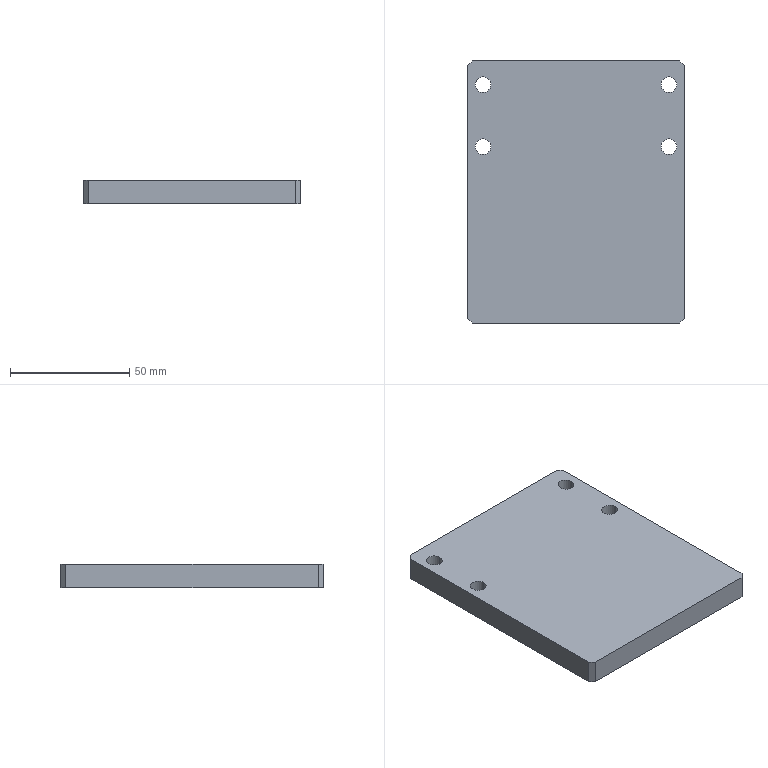Part | SolidWorks | features BaseBody 1 | 1 solid | 18 faces | box 91 x 110 x 10 mm | volume 98652 mm3 | plane 10 | cylinder 8 | commonest cylinder face diameters 6.6 x8
STEP:
#1=CARTESIAN_POINT('',(-42.3,19.,0.));
#2=VERTEX_POINT('',#1);
#3=CARTESIAN_POINT('',(-35.7,19.,0.));
#4=VERTEX_POINT('',#3);
#5=CARTESIAN_POINT('',(-39.,19.,0.));
#6=DIRECTION('',(0.,0.,1.));
#7=DIRECTION('',(1.,0.,0.));
#8=AXIS2_PLACEMENT_3D('',#5,#6,#7);
#9=CIRCLE('',#8,3.3);
#10=EDGE_CURVE('',#2,#4,#9,.T.);
#11=ORIENTED_EDGE('',*,*,#10,.F.);
#12=CARTESIAN_POINT('',(-42.3,19.,10.));
#13=VERTEX_POINT('',#12);
#14=CARTESIAN_POINT('',(-42.3,19.,10.));
#15=DIRECTION('',(0.,0.,1.));
#16=VECTOR('',#15,1000.);
#17=LINE('',#14,#16);
#18=EDGE_CURVE('',#2,#13,#17,.T.);
#19=ORIENTED_EDGE('',*,*,#18,.T.);
#20=CARTESIAN_POINT('',(-35.7,19.,10.));
#21=VERTEX_POINT('',#20);
#22=CARTESIAN_POINT('',(-39.,19.,10.));
#23=DIRECTION('',(0.,0.,-1.));
#24=DIRECTION('',(1.,0.,0.));
#25=AXIS2_PLACEMENT_3D('',#22,#23,#24);
#26=CIRCLE('',#25,3.3);
#27=EDGE_CURVE('',#21,#13,#26,.T.);
#28=ORIENTED_EDGE('',*,*,#27,.F.);
#29=CARTESIAN_POINT('',(-35.7,19.,10.));
#30=DIRECTION('',(0.,0.,1.));
#31=VECTOR('',#30,1000.);
#32=LINE('',#29,#31);
#33=EDGE_CURVE('',#4,#21,#32,.T.);
#34=ORIENTED_EDGE('',*,*,#33,.F.);
#35=EDGE_LOOP('',(#11,#19,#28,#34));
#36=FACE_OUTER_BOUND('',#35,.T.);
#37=CARTESIAN_POINT('',(-39.,19.,10.));
#38=DIRECTION('',(0.,0.,1.));
#39=DIRECTION('',(1.,0.,0.));
#40=AXIS2_PLACEMENT_3D('',#37,#38,#39);
#41=CYLINDRICAL_SURFACE('',#40,3.3);
#42=ADVANCED_FACE('',(#36),#41,.F.);
#43=CARTESIAN_POINT('',(35.7,19.,0.));
#44=VERTEX_POINT('',#43);
#45=CARTESIAN_POINT('',(42.3,19.,0.));
#46=VERTEX_POINT('',#45);
#47=CARTESIAN_POINT('',(39.,19.,0.));
#48=DIRECTION('',(0.,0.,1.));
#49=DIRECTION('',(1.,0.,0.));
#50=AXIS2_PLACEMENT_3D('',#47,#48,#49);
#51=CIRCLE('',#50,3.3);
#52=EDGE_CURVE('',#44,#46,#51,.T.);
#53=ORIENTED_EDGE('',*,*,#52,.F.);
#54=CARTESIAN_POINT('',(35.7,19.,10.));
#55=VERTEX_POINT('',#54);
#56=CARTESIAN_POINT('',(35.7,19.,10.));
#57=DIRECTION('',(0.,0.,1.));
#58=VECTOR('',#57,1000.);
#59=LINE('',#56,#58);
#60=EDGE_CURVE('',#44,#55,#59,.T.);
#61=ORIENTED_EDGE('',*,*,#60,.T.);
#62=CARTESIAN_POINT('',(42.3,19.,10.));
#63=VERTEX_POINT('',#62);
#64=CARTESIAN_POINT('',(39.,19.,10.));
#65=DIRECTION('',(0.,0.,-1.));
#66=DIRECTION('',(1.,0.,0.));
#67=AXIS2_PLACEMENT_3D('',#64,#65,#66);
#68=CIRCLE('',#67,3.3);
#69=EDGE_CURVE('',#63,#55,#68,.T.);
#70=ORIENTED_EDGE('',*,*,#69,.F.);
#71=CARTESIAN_POINT('',(42.3,19.,10.));
#72=DIRECTION('',(0.,0.,1.));
#73=VECTOR('',#72,1000.);
#74=LINE('',#71,#73);
#75=EDGE_CURVE('',#46,#63,#74,.T.);
#76=ORIENTED_EDGE('',*,*,#75,.F.);
#77=EDGE_LOOP('',(#53,#61,#70,#76));
#78=FACE_OUTER_BOUND('',#77,.T.);
#79=CARTESIAN_POINT('',(39.,19.,10.));
#80=DIRECTION('',(0.,0.,1.));
#81=DIRECTION('',(1.,0.,0.));
#82=AXIS2_PLACEMENT_3D('',#79,#80,#81);
#83=CYLINDRICAL_SURFACE('',#82,3.3);
#84=ADVANCED_FACE('',(#78),#83,.F.);
#85=CARTESIAN_POINT('',(35.7,45.,0.));
#86=VERTEX_POINT('',#85);
#87=CARTESIAN_POINT('',(42.3,45.,0.));
#88=VERTEX_POINT('',#87);
#89=CARTESIAN_POINT('',(39.,45.,0.));
#90=DIRECTION('',(0.,0.,1.));
#91=DIRECTION('',(1.,0.,0.));
#92=AXIS2_PLACEMENT_3D('',#89,#90,#91);
#93=CIRCLE('',#92,3.3);
#94=EDGE_CURVE('',#86,#88,#93,.T.);
#95=ORIENTED_EDGE('',*,*,#94,.F.);
#96=CARTESIAN_POINT('',(35.7,45.,10.));
#97=VERTEX_POINT('',#96);
#98=CARTESIAN_POINT('',(35.7,45.,10.));
#99=DIRECTION('',(0.,0.,1.));
#100=VECTOR('',#99,1000.);
#101=LINE('',#98,#100);
#102=EDGE_CURVE('',#86,#97,#101,.T.);
#103=ORIENTED_EDGE('',*,*,#102,.T.);
#104=CARTESIAN_POINT('',(42.3,45.,10.));
#105=VERTEX_POINT('',#104);
#106=CARTESIAN_POINT('',(39.,45.,10.));
#107=DIRECTION('',(0.,0.,-1.));
#108=DIRECTION('',(1.,0.,0.));
#109=AXIS2_PLACEMENT_3D('',#106,#107,#108);
#110=CIRCLE('',#109,3.3);
#111=EDGE_CURVE('',#105,#97,#110,.T.);
#112=ORIENTED_EDGE('',*,*,#111,.F.);
#113=CARTESIAN_POINT('',(42.3,45.,10.));
#114=DIRECTION('',(0.,0.,1.));
#115=VECTOR('',#114,1000.);
#116=LINE('',#113,#115);
#117=EDGE_CURVE('',#88,#105,#116,.T.);
#118=ORIENTED_EDGE('',*,*,#117,.F.);
#119=EDGE_LOOP('',(#95,#103,#112,#118));
#120=FACE_OUTER_BOUND('',#119,.T.);
#121=CARTESIAN_POINT('',(39.,45.,10.));
#122=DIRECTION('',(0.,0.,1.));
#123=DIRECTION('',(1.,0.,0.));
#124=AXIS2_PLACEMENT_3D('',#121,#122,#123);
#125=CYLINDRICAL_SURFACE('',#124,3.3);
#126=ADVANCED_FACE('',(#120),#125,.F.);
#127=CARTESIAN_POINT('',(-42.3,45.,0.));
#128=VERTEX_POINT('',#127);
#129=CARTESIAN_POINT('',(-35.7,45.,0.));
#130=VERTEX_POINT('',#129);
#131=CARTESIAN_POINT('',(-39.,45.,0.));
#132=DIRECTION('',(0.,0.,1.));
#133=DIRECTION('',(1.,0.,0.));
#134=AXIS2_PLACEMENT_3D('',#131,#132,#133);
#135=CIRCLE('',#134,3.3);
#136=EDGE_CURVE('',#128,#130,#135,.T.);
#137=ORIENTED_EDGE('',*,*,#136,.F.);
#138=CARTESIAN_POINT('',(-42.3,45.,10.));
#139=VERTEX_POINT('',#138);
#140=CARTESIAN_POINT('',(-42.3,45.,10.));
#141=DIRECTION('',(0.,0.,1.));
#142=VECTOR('',#141,1000.);
#143=LINE('',#140,#142);
#144=EDGE_CURVE('',#128,#139,#143,.T.);
#145=ORIENTED_EDGE('',*,*,#144,.T.);
#146=CARTESIAN_POINT('',(-35.7,45.,10.));
#147=VERTEX_POINT('',#146);
#148=CARTESIAN_POINT('',(-39.,45.,10.));
#149=DIRECTION('',(0.,0.,-1.));
#150=DIRECTION('',(1.,0.,0.));
#151=AXIS2_PLACEMENT_3D('',#148,#149,#150);
#152=CIRCLE('',#151,3.3);
#153=EDGE_CURVE('',#147,#139,#152,.T.);
#154=ORIENTED_EDGE('',*,*,#153,.F.);
#155=CARTESIAN_POINT('',(-35.7,45.,10.));
#156=DIRECTION('',(0.,0.,1.));
#157=VECTOR('',#156,1000.);
#158=LINE('',#155,#157);
#159=EDGE_CURVE('',#130,#147,#158,.T.);
#160=ORIENTED_EDGE('',*,*,#159,.F.);
#161=EDGE_LOOP('',(#137,#145,#154,#160));
#162=FACE_OUTER_BOUND('',#161,.T.);
#163=CARTESIAN_POINT('',(-39.,45.,10.));
#164=DIRECTION('',(0.,0.,1.));
#165=DIRECTION('',(1.,0.,0.));
#166=AXIS2_PLACEMENT_3D('',#163,#164,#165);
#167=CYLINDRICAL_SURFACE('',#166,3.3);
#168=ADVANCED_FACE('',(#162),#167,.F.);
#169=CARTESIAN_POINT('',(43.5,55.,10.));
#170=VERTEX_POINT('',#169);
#171=CARTESIAN_POINT('',(-43.5,55.,10.));
#172=VERTEX_POINT('',#171);
#173=CARTESIAN_POINT('',(0.,55.,10.));
#174=DIRECTION('',(-1.,0.,0.));
#175=VECTOR('',#174,1000.);
#176=LINE('',#173,#175);
#177=EDGE_CURVE('',#170,#172,#176,.T.);
#178=ORIENTED_EDGE('',*,*,#177,.T.);
#179=CARTESIAN_POINT('',(-45.5,53.,10.));
#180=VERTEX_POINT('',#179);
#181=CARTESIAN_POINT('',(-43.5,55.,10.));
#182=DIRECTION('',(-0.7071,-0.7071,0.));
#183=VECTOR('',#182,1000.);
#184=LINE('',#181,#183);
#185=EDGE_CURVE('',#172,#180,#184,.T.);
#186=ORIENTED_EDGE('',*,*,#185,.T.);
#187=CARTESIAN_POINT('',(-45.5,-53.,10.));
#188=VERTEX_POINT('',#187);
#189=CARTESIAN_POINT('',(-45.5,0.,10.));
#190=DIRECTION('',(0.,-1.,0.));
#191=VECTOR('',#190,1000.);
#192=LINE('',#189,#191);
#193=EDGE_CURVE('',#180,#188,#192,.T.);
#194=ORIENTED_EDGE('',*,*,#193,.T.);
#195=CARTESIAN_POINT('',(-43.5,-55.,10.));
#196=VERTEX_POINT('',#195);
#197=CARTESIAN_POINT('',(-45.5,-53.,10.));
#198=DIRECTION('',(0.7071,-0.7071,0.));
#199=VECTOR('',#198,1000.);
#200=LINE('',#197,#199);
#201=EDGE_CURVE('',#188,#196,#200,.T.);
#202=ORIENTED_EDGE('',*,*,#201,.T.);
#203=CARTESIAN_POINT('',(43.5,-55.,10.));
#204=VERTEX_POINT('',#203);
#205=CARTESIAN_POINT('',(0.,-55.,10.));
#206=DIRECTION('',(1.,0.,0.));
#207=VECTOR('',#206,1000.);
#208=LINE('',#205,#207);
#209=EDGE_CURVE('',#196,#204,#208,.T.);
#210=ORIENTED_EDGE('',*,*,#209,.T.);
#211=CARTESIAN_POINT('',(45.5,-53.,10.));
#212=VERTEX_POINT('',#211);
#213=CARTESIAN_POINT('',(43.5,-55.,10.));
#214=DIRECTION('',(0.7071,0.7071,0.));
#215=VECTOR('',#214,1000.);
#216=LINE('',#213,#215);
#217=EDGE_CURVE('',#204,#212,#216,.T.);
#218=ORIENTED_EDGE('',*,*,#217,.T.);
#219=CARTESIAN_POINT('',(45.5,53.,10.));
#220=VERTEX_POINT('',#219);
#221=CARTESIAN_POINT('',(45.5,0.,10.));
#222=DIRECTION('',(0.,1.,0.));
#223=VECTOR('',#222,1000.);
#224=LINE('',#221,#223);
#225=EDGE_CURVE('',#212,#220,#224,.T.);
#226=ORIENTED_EDGE('',*,*,#225,.T.);
#227=CARTESIAN_POINT('',(45.5,53.,10.));
#228=DIRECTION('',(-0.7071,0.7071,0.));
#229=VECTOR('',#228,1000.);
#230=LINE('',#227,#229);
#231=EDGE_CURVE('',#220,#170,#230,.T.);
#232=ORIENTED_EDGE('',*,*,#231,.T.);
#233=EDGE_LOOP('',(#178,#186,#194,#202,#210,#218,#226,#232));
#234=FACE_OUTER_BOUND('',#233,.T.);
#235=ORIENTED_EDGE('',*,*,#27,.T.);
#236=CARTESIAN_POINT('',(-39.,19.,10.));
#237=DIRECTION('',(0.,0.,-1.));
#238=DIRECTION('',(1.,0.,0.));
#239=AXIS2_PLACEMENT_3D('',#236,#237,#238);
#240=CIRCLE('',#239,3.3);
#241=EDGE_CURVE('',#13,#21,#240,.T.);
#242=ORIENTED_EDGE('',*,*,#241,.T.);
#243=EDGE_LOOP('',(#235,#242));
#244=FACE_BOUND('',#243,.T.);
#245=ORIENTED_EDGE('',*,*,#69,.T.);
#246=CARTESIAN_POINT('',(39.,19.,10.));
#247=DIRECTION('',(0.,0.,-1.));
#248=DIRECTION('',(1.,0.,0.));
#249=AXIS2_PLACEMENT_3D('',#246,#247,#248);
#250=CIRCLE('',#249,3.3);
#251=EDGE_CURVE('',#55,#63,#250,.T.);
#252=ORIENTED_EDGE('',*,*,#251,.T.);
#253=EDGE_LOOP('',(#245,#252));
#254=FACE_BOUND('',#253,.T.);
#255=ORIENTED_EDGE('',*,*,#111,.T.);
#256=CARTESIAN_POINT('',(39.,45.,10.));
#257=DIRECTION('',(0.,0.,-1.));
#258=DIRECTION('',(1.,0.,0.));
#259=AXIS2_PLACEMENT_3D('',#256,#257,#258);
#260=CIRCLE('',#259,3.3);
#261=EDGE_CURVE('',#97,#105,#260,.T.);
#262=ORIENTED_EDGE('',*,*,#261,.T.);
#263=EDGE_LOOP('',(#255,#262));
#264=FACE_BOUND('',#263,.T.);
#265=ORIENTED_EDGE('',*,*,#153,.T.);
#266=CARTESIAN_POINT('',(-39.,45.,10.));
#267=DIRECTION('',(0.,0.,-1.));
#268=DIRECTION('',(1.,0.,0.));
#269=AXIS2_PLACEMENT_3D('',#266,#267,#268);
#270=CIRCLE('',#269,3.3);
#271=EDGE_CURVE('',#139,#147,#270,.T.);
#272=ORIENTED_EDGE('',*,*,#271,.T.);
#273=EDGE_LOOP('',(#265,#272));
#274=FACE_BOUND('',#273,.T.);
#275=CARTESIAN_POINT('',(0.,0.,10.));
#276=DIRECTION('',(0.,0.,1.));
#277=DIRECTION('',(1.,0.,0.));
#278=AXIS2_PLACEMENT_3D('',#275,#276,#277);
#279=PLANE('',#278);
#280=ADVANCED_FACE('',(#234,#244,#254,#264,#274),#279,.T.);
#281=CARTESIAN_POINT('',(-43.5,55.,0.));
#282=VERTEX_POINT('',#281);
#283=CARTESIAN_POINT('',(-43.5,55.,10.));
#284=DIRECTION('',(0.,0.,1.));
#285=VECTOR('',#284,1000.);
#286=LINE('',#283,#285);
#287=EDGE_CURVE('',#282,#172,#286,.T.);
#288=ORIENTED_EDGE('',*,*,#287,.F.);
#289=CARTESIAN_POINT('',(-45.5,53.,0.));
#290=VERTEX_POINT('',#289);
#291=CARTESIAN_POINT('',(-45.5,53.,0.));
#292=DIRECTION('',(0.7071,0.7071,0.));
#293=VECTOR('',#292,1000.);
#294=LINE('',#291,#293);
#295=EDGE_CURVE('',#290,#282,#294,.T.);
#296=ORIENTED_EDGE('',*,*,#295,.F.);
#297=CARTESIAN_POINT('',(-45.5,53.,10.));
#298=DIRECTION('',(0.,0.,-1.));
#299=VECTOR('',#298,1000.);
#300=LINE('',#297,#299);
#301=EDGE_CURVE('',#180,#290,#300,.T.);
#302=ORIENTED_EDGE('',*,*,#301,.F.);
#303=ORIENTED_EDGE('',*,*,#185,.F.);
#304=EDGE_LOOP('',(#288,#296,#302,#303));
#305=FACE_OUTER_BOUND('',#304,.T.);
#306=CARTESIAN_POINT('',(-45.5,53.,10.));
#307=DIRECTION('',(0.7071,-0.7071,0.));
#308=DIRECTION('',(0.7071,0.7071,0.));
#309=AXIS2_PLACEMENT_3D('',#306,#307,#308);
#310=PLANE('',#309);
#311=ADVANCED_FACE('',(#305),#310,.F.);
#312=CARTESIAN_POINT('',(43.5,55.,0.));
#313=VERTEX_POINT('',#312);
#314=CARTESIAN_POINT('',(43.5,55.,10.));
#315=DIRECTION('',(0.,0.,1.));
#316=VECTOR('',#315,1000.);
#317=LINE('',#314,#316);
#318=EDGE_CURVE('',#313,#170,#317,.T.);
#319=ORIENTED_EDGE('',*,*,#318,.F.);
#320=CARTESIAN_POINT('',(-45.5,55.,0.));
#321=DIRECTION('',(1.,0.,0.));
#322=VECTOR('',#321,1000.);
#323=LINE('',#320,#322);
#324=EDGE_CURVE('',#282,#313,#323,.T.);
#325=ORIENTED_EDGE('',*,*,#324,.F.);
#326=ORIENTED_EDGE('',*,*,#287,.T.);
#327=ORIENTED_EDGE('',*,*,#177,.F.);
#328=EDGE_LOOP('',(#319,#325,#326,#327));
#329=FACE_OUTER_BOUND('',#328,.T.);
#330=CARTESIAN_POINT('',(-45.5,55.,10.));
#331=DIRECTION('',(0.,-1.,0.));
#332=DIRECTION('',(0.,0.,-1.));
#333=AXIS2_PLACEMENT_3D('',#330,#331,#332);
#334=PLANE('',#333);
#335=ADVANCED_FACE('',(#329),#334,.F.);
#336=CARTESIAN_POINT('',(45.5,53.,0.));
#337=VERTEX_POINT('',#336);
#338=CARTESIAN_POINT('',(45.5,53.,10.));
#339=DIRECTION('',(0.,0.,1.));
#340=VECTOR('',#339,1000.);
#341=LINE('',#338,#340);
#342=EDGE_CURVE('',#337,#220,#341,.T.);
#343=ORIENTED_EDGE('',*,*,#342,.F.);
#344=CARTESIAN_POINT('',(43.5,55.,0.));
#345=DIRECTION('',(0.7071,-0.7071,0.));
#346=VECTOR('',#345,1000.);
#347=LINE('',#344,#346);
#348=EDGE_CURVE('',#313,#337,#347,.T.);
#349=ORIENTED_EDGE('',*,*,#348,.F.);
#350=ORIENTED_EDGE('',*,*,#318,.T.);
#351=ORIENTED_EDGE('',*,*,#231,.F.);
#352=EDGE_LOOP('',(#343,#349,#350,#351));
#353=FACE_OUTER_BOUND('',#352,.T.);
#354=CARTESIAN_POINT('',(43.5,55.,10.));
#355=DIRECTION('',(-0.7071,-0.7071,0.));
#356=DIRECTION('',(0.7071,-0.7071,0.));
#357=AXIS2_PLACEMENT_3D('',#354,#355,#356);
#358=PLANE('',#357);
#359=ADVANCED_FACE('',(#353),#358,.F.);
#360=CARTESIAN_POINT('',(45.5,-53.,0.));
#361=VERTEX_POINT('',#360);
#362=CARTESIAN_POINT('',(45.5,-53.,10.));
#363=DIRECTION('',(0.,0.,1.));
#364=VECTOR('',#363,1000.);
#365=LINE('',#362,#364);
#366=EDGE_CURVE('',#361,#212,#365,.T.);
#367=ORIENTED_EDGE('',*,*,#366,.F.);
#368=CARTESIAN_POINT('',(45.5,55.,0.));
#369=DIRECTION('',(0.,-1.,0.));
#370=VECTOR('',#369,1000.);
#371=LINE('',#368,#370);
#372=EDGE_CURVE('',#337,#361,#371,.T.);
#373=ORIENTED_EDGE('',*,*,#372,.F.);
#374=ORIENTED_EDGE('',*,*,#342,.T.);
#375=ORIENTED_EDGE('',*,*,#225,.F.);
#376=EDGE_LOOP('',(#367,#373,#374,#375));
#377=FACE_OUTER_BOUND('',#376,.T.);
#378=CARTESIAN_POINT('',(45.5,55.,10.));
#379=DIRECTION('',(-1.,0.,0.));
#380=DIRECTION('',(0.,-1.,0.));
#381=AXIS2_PLACEMENT_3D('',#378,#379,#380);
#382=PLANE('',#381);
#383=ADVANCED_FACE('',(#377),#382,.F.);
#384=CARTESIAN_POINT('',(43.5,-55.,0.));
#385=VERTEX_POINT('',#384);
#386=CARTESIAN_POINT('',(43.5,-55.,10.));
#387=DIRECTION('',(0.,0.,1.));
#388=VECTOR('',#387,1000.);
#389=LINE('',#386,#388);
#390=EDGE_CURVE('',#385,#204,#389,.T.);
#391=ORIENTED_EDGE('',*,*,#390,.F.);
#392=CARTESIAN_POINT('',(45.5,-53.,0.));
#393=DIRECTION('',(-0.7071,-0.7071,0.));
#394=VECTOR('',#393,1000.);
#395=LINE('',#392,#394);
#396=EDGE_CURVE('',#361,#385,#395,.T.);
#397=ORIENTED_EDGE('',*,*,#396,.F.);
#398=ORIENTED_EDGE('',*,*,#366,.T.);
#399=ORIENTED_EDGE('',*,*,#217,.F.);
#400=EDGE_LOOP('',(#391,#397,#398,#399));
#401=FACE_OUTER_BOUND('',#400,.T.);
#402=CARTESIAN_POINT('',(45.5,-53.,10.));
#403=DIRECTION('',(-0.7071,0.7071,0.));
#404=DIRECTION('',(-0.7071,-0.7071,0.));
#405=AXIS2_PLACEMENT_3D('',#402,#403,#404);
#406=PLANE('',#405);
#407=ADVANCED_FACE('',(#401),#406,.F.);
#408=CARTESIAN_POINT('',(-43.5,-55.,0.));
#409=VERTEX_POINT('',#408);
#410=CARTESIAN_POINT('',(-43.5,-55.,10.));
#411=DIRECTION('',(0.,0.,1.));
#412=VECTOR('',#411,1000.);
#413=LINE('',#410,#412);
#414=EDGE_CURVE('',#409,#196,#413,.T.);
#415=ORIENTED_EDGE('',*,*,#414,.F.);
#416=CARTESIAN_POINT('',(-45.5,-55.,0.));
#417=DIRECTION('',(-1.,0.,0.));
#418=VECTOR('',#417,1000.);
#419=LINE('',#416,#418);
#420=EDGE_CURVE('',#385,#409,#419,.T.);
#421=ORIENTED_EDGE('',*,*,#420,.F.);
#422=ORIENTED_EDGE('',*,*,#390,.T.);
#423=ORIENTED_EDGE('',*,*,#209,.F.);
#424=EDGE_LOOP('',(#415,#421,#422,#423));
#425=FACE_OUTER_BOUND('',#424,.T.);
#426=CARTESIAN_POINT('',(-45.5,-55.,10.));
#427=DIRECTION('',(0.,1.,0.));
#428=DIRECTION('',(0.,0.,1.));
#429=AXIS2_PLACEMENT_3D('',#426,#427,#428);
#430=PLANE('',#429);
#431=ADVANCED_FACE('',(#425),#430,.F.);
#432=CARTESIAN_POINT('',(-45.5,-53.,0.));
#433=VERTEX_POINT('',#432);
#434=CARTESIAN_POINT('',(-45.5,-53.,10.));
#435=DIRECTION('',(0.,0.,1.));
#436=VECTOR('',#435,1000.);
#437=LINE('',#434,#436);
#438=EDGE_CURVE('',#433,#188,#437,.T.);
#439=ORIENTED_EDGE('',*,*,#438,.F.);
#440=CARTESIAN_POINT('',(-43.5,-55.,0.));
#441=DIRECTION('',(-0.7071,0.7071,0.));
#442=VECTOR('',#441,1000.);
#443=LINE('',#440,#442);
#444=EDGE_CURVE('',#409,#433,#443,.T.);
#445=ORIENTED_EDGE('',*,*,#444,.F.);
#446=ORIENTED_EDGE('',*,*,#414,.T.);
#447=ORIENTED_EDGE('',*,*,#201,.F.);
#448=EDGE_LOOP('',(#439,#445,#446,#447));
#449=FACE_OUTER_BOUND('',#448,.T.);
#450=CARTESIAN_POINT('',(-43.5,-55.,10.));
#451=DIRECTION('',(0.7071,0.7071,0.));
#452=DIRECTION('',(-0.7071,0.7071,0.));
#453=AXIS2_PLACEMENT_3D('',#450,#451,#452);
#454=PLANE('',#453);
#455=ADVANCED_FACE('',(#449),#454,.F.);
#456=ORIENTED_EDGE('',*,*,#438,.T.);
#457=ORIENTED_EDGE('',*,*,#193,.F.);
#458=ORIENTED_EDGE('',*,*,#301,.T.);
#459=CARTESIAN_POINT('',(-45.5,55.,0.));
#460=DIRECTION('',(0.,1.,0.));
#461=VECTOR('',#460,1000.);
#462=LINE('',#459,#461);
#463=EDGE_CURVE('',#433,#290,#462,.T.);
#464=ORIENTED_EDGE('',*,*,#463,.F.);
#465=EDGE_LOOP('',(#456,#457,#458,#464));
#466=FACE_OUTER_BOUND('',#465,.T.);
#467=CARTESIAN_POINT('',(-45.5,55.,10.));
#468=DIRECTION('',(1.,0.,0.));
#469=DIRECTION('',(0.,1.,0.));
#470=AXIS2_PLACEMENT_3D('',#467,#468,#469);
#471=PLANE('',#470);
#472=ADVANCED_FACE('',(#466),#471,.F.);
#473=ORIENTED_EDGE('',*,*,#18,.F.);
#474=CARTESIAN_POINT('',(-39.,19.,0.));
#475=DIRECTION('',(0.,0.,1.));
#476=DIRECTION('',(1.,0.,0.));
#477=AXIS2_PLACEMENT_3D('',#474,#475,#476);
#478=CIRCLE('',#477,3.3);
#479=EDGE_CURVE('',#4,#2,#478,.T.);
#480=ORIENTED_EDGE('',*,*,#479,.F.);
#481=ORIENTED_EDGE('',*,*,#33,.T.);
#482=ORIENTED_EDGE('',*,*,#241,.F.);
#483=EDGE_LOOP('',(#473,#480,#481,#482));
#484=FACE_OUTER_BOUND('',#483,.T.);
#485=CARTESIAN_POINT('',(-39.,19.,10.));
#486=DIRECTION('',(0.,0.,1.));
#487=DIRECTION('',(1.,0.,0.));
#488=AXIS2_PLACEMENT_3D('',#485,#486,#487);
#489=CYLINDRICAL_SURFACE('',#488,3.3);
#490=ADVANCED_FACE('',(#484),#489,.F.);
#491=ORIENTED_EDGE('',*,*,#60,.F.);
#492=CARTESIAN_POINT('',(39.,19.,0.));
#493=DIRECTION('',(0.,0.,1.));
#494=DIRECTION('',(1.,0.,0.));
#495=AXIS2_PLACEMENT_3D('',#492,#493,#494);
#496=CIRCLE('',#495,3.3);
#497=EDGE_CURVE('',#46,#44,#496,.T.);
#498=ORIENTED_EDGE('',*,*,#497,.F.);
#499=ORIENTED_EDGE('',*,*,#75,.T.);
#500=ORIENTED_EDGE('',*,*,#251,.F.);
#501=EDGE_LOOP('',(#491,#498,#499,#500));
#502=FACE_OUTER_BOUND('',#501,.T.);
#503=CARTESIAN_POINT('',(39.,19.,10.));
#504=DIRECTION('',(0.,0.,1.));
#505=DIRECTION('',(1.,0.,0.));
#506=AXIS2_PLACEMENT_3D('',#503,#504,#505);
#507=CYLINDRICAL_SURFACE('',#506,3.3);
#508=ADVANCED_FACE('',(#502),#507,.F.);
#509=ORIENTED_EDGE('',*,*,#102,.F.);
#510=CARTESIAN_POINT('',(39.,45.,0.));
#511=DIRECTION('',(0.,0.,1.));
#512=DIRECTION('',(1.,0.,0.));
#513=AXIS2_PLACEMENT_3D('',#510,#511,#512);
#514=CIRCLE('',#513,3.3);
#515=EDGE_CURVE('',#88,#86,#514,.T.);
#516=ORIENTED_EDGE('',*,*,#515,.F.);
#517=ORIENTED_EDGE('',*,*,#117,.T.);
#518=ORIENTED_EDGE('',*,*,#261,.F.);
#519=EDGE_LOOP('',(#509,#516,#517,#518));
#520=FACE_OUTER_BOUND('',#519,.T.);
#521=CARTESIAN_POINT('',(39.,45.,10.));
#522=DIRECTION('',(0.,0.,1.));
#523=DIRECTION('',(1.,0.,0.));
#524=AXIS2_PLACEMENT_3D('',#521,#522,#523);
#525=CYLINDRICAL_SURFACE('',#524,3.3);
#526=ADVANCED_FACE('',(#520),#525,.F.);
#527=ORIENTED_EDGE('',*,*,#144,.F.);
#528=CARTESIAN_POINT('',(-39.,45.,0.));
#529=DIRECTION('',(0.,0.,1.));
#530=DIRECTION('',(1.,0.,0.));
#531=AXIS2_PLACEMENT_3D('',#528,#529,#530);
#532=CIRCLE('',#531,3.3);
#533=EDGE_CURVE('',#130,#128,#532,.T.);
#534=ORIENTED_EDGE('',*,*,#533,.F.);
#535=ORIENTED_EDGE('',*,*,#159,.T.);
#536=ORIENTED_EDGE('',*,*,#271,.F.);
#537=EDGE_LOOP('',(#527,#534,#535,#536));
#538=FACE_OUTER_BOUND('',#537,.T.);
#539=CARTESIAN_POINT('',(-39.,45.,10.));
#540=DIRECTION('',(0.,0.,1.));
#541=DIRECTION('',(1.,0.,0.));
#542=AXIS2_PLACEMENT_3D('',#539,#540,#541);
#543=CYLINDRICAL_SURFACE('',#542,3.3);
#544=ADVANCED_FACE('',(#538),#543,.F.);
#545=ORIENTED_EDGE('',*,*,#444,.T.);
#546=ORIENTED_EDGE('',*,*,#463,.T.);
#547=ORIENTED_EDGE('',*,*,#295,.T.);
#548=ORIENTED_EDGE('',*,*,#324,.T.);
#549=ORIENTED_EDGE('',*,*,#348,.T.);
#550=ORIENTED_EDGE('',*,*,#372,.T.);
#551=ORIENTED_EDGE('',*,*,#396,.T.);
#552=ORIENTED_EDGE('',*,*,#420,.T.);
#553=EDGE_LOOP('',(#545,#546,#547,#548,#549,#550,#551,#552));
#554=FACE_OUTER_BOUND('',#553,.T.);
#555=ORIENTED_EDGE('',*,*,#479,.T.);
#556=ORIENTED_EDGE('',*,*,#10,.T.);
#557=EDGE_LOOP('',(#555,#556));
#558=FACE_BOUND('',#557,.T.);
#559=ORIENTED_EDGE('',*,*,#497,.T.);
#560=ORIENTED_EDGE('',*,*,#52,.T.);
#561=EDGE_LOOP('',(#559,#560));
#562=FACE_BOUND('',#561,.T.);
#563=ORIENTED_EDGE('',*,*,#515,.T.);
#564=ORIENTED_EDGE('',*,*,#94,.T.);
#565=EDGE_LOOP('',(#563,#564));
#566=FACE_BOUND('',#565,.T.);
#567=ORIENTED_EDGE('',*,*,#533,.T.);
#568=ORIENTED_EDGE('',*,*,#136,.T.);
#569=EDGE_LOOP('',(#567,#568));
#570=FACE_BOUND('',#569,.T.);
#571=CARTESIAN_POINT('',(0.,0.,0.));
#572=DIRECTION('',(0.,0.,1.));
#573=DIRECTION('',(1.,0.,0.));
#574=AXIS2_PLACEMENT_3D('',#571,#572,#573);
#575=PLANE('',#574);
#576=ADVANCED_FACE('',(#554,#558,#562,#566,#570),#575,.F.);
#577=CLOSED_SHELL('',(#42,#84,#126,#168,#280,#311,#335,#359,#383,#407,#431,#455,#472,#490,#508,#526,#544,#576));
#578=MANIFOLD_SOLID_BREP('',#577);
#579=CARTESIAN_POINT('',(0.,0.,0.));
#580=DIRECTION('',(0.,0.,1.));
#581=DIRECTION('',(1.,0.,0.));
#582=AXIS2_PLACEMENT_3D('',#579,#580,#581);
#583=(LENGTH_UNIT()NAMED_UNIT(*)SI_UNIT(.MILLI.,.METRE.));
#584=UNCERTAINTY_MEASURE_WITH_UNIT(LENGTH_MEASURE(0.00001),#583,'','');
#585=(NAMED_UNIT(*)PLANE_ANGLE_UNIT()SI_UNIT($,.RADIAN.));
#586=(NAMED_UNIT(*)SI_UNIT($,.STERADIAN.)SOLID_ANGLE_UNIT());
#587=(GEOMETRIC_REPRESENTATION_CONTEXT(3)GLOBAL_UNCERTAINTY_ASSIGNED_CONTEXT((#584))GLOBAL_UNIT_ASSIGNED_CONTEXT((#583,#585,#586))REPRESENTATION_CONTEXT('',''));
#588=ADVANCED_BREP_SHAPE_REPRESENTATION('',(#578,#582),#587);